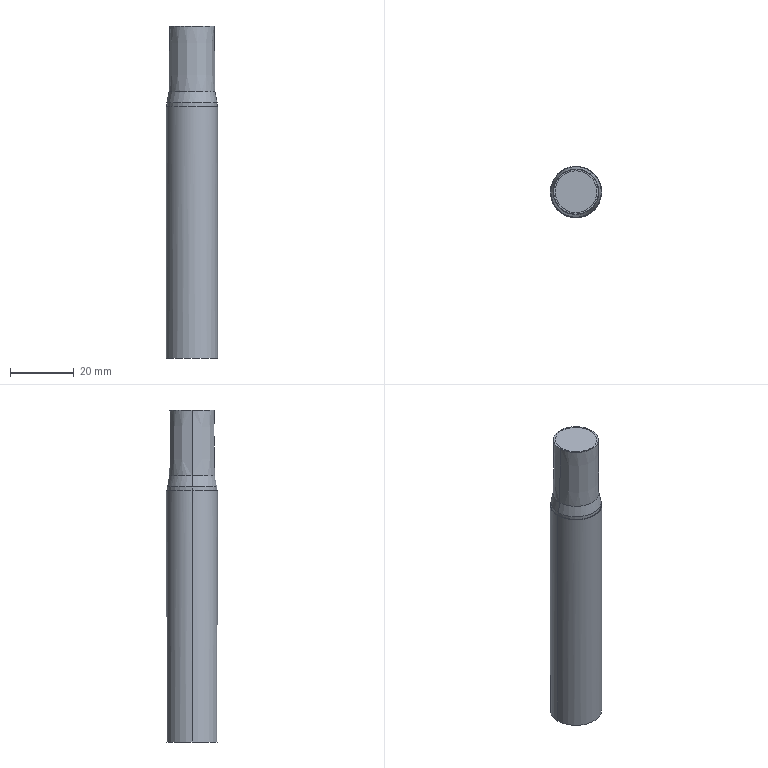Part | Creo | 1 solid | 15 faces | box 16 x 16 x 103.751 mm | volume 19849 mm3 | plane 7 | cone 4 | cylinder 4 | commonest cylinder face diameters 15.678 x2 16 x2
STEP:
#1=CARTESIAN_POINT('',(0.,0.,0.));
#2=DIRECTION('',(0.,0.,1.));
#3=DIRECTION('',(1.,0.,0.));
#4=AXIS2_PLACEMENT_3D('',#1,#2,#3);
#5=CARTESIAN_POINT('',(-38.231,-245.907,-49.693));
#6=VERTEX_POINT('',#5);
#7=CARTESIAN_POINT('',(-31.681,-252.457,-49.728));
#8=VERTEX_POINT('',#7);
#9=CARTESIAN_POINT('',(-37.799,-245.909,-49.693));
#10=CARTESIAN_POINT('',(-36.952,-245.993,-49.694));
#11=CARTESIAN_POINT('',(-35.715,-246.368,-49.696));
#12=CARTESIAN_POINT('',(-34.571,-246.974,-49.699));
#13=CARTESIAN_POINT('',(-33.563,-247.793,-49.703));
#14=CARTESIAN_POINT('',(-32.745,-248.801,-49.709));
#15=CARTESIAN_POINT('',(-32.141,-249.945,-49.715));
#16=CARTESIAN_POINT('',(-31.766,-251.181,-49.721));
#17=CARTESIAN_POINT('',(-31.682,-252.026,-49.726));
#18=B_SPLINE_CURVE_WITH_KNOTS('',3,(#5,#9,#10,#11,#12,#13,#14,#15,#16,#17,#7),.UNSPECIFIED.,.F.,.F.,(4,1,1,1,1,1,1,1,4),(0.,0.125,0.25,0.375,0.5,0.625,0.75,0.875,1.),.UNSPECIFIED.);
#19=EDGE_CURVE('',#6,#8,#18,.T.);
#20=ORIENTED_EDGE('',*,*,#19,.T.);
#21=CARTESIAN_POINT('',(-38.231,-259.008,-49.763));
#22=VERTEX_POINT('',#21);
#23=CARTESIAN_POINT('',(-31.681,-252.457,-49.728));
#24=CARTESIAN_POINT('',(-31.682,-252.889,-49.731));
#25=CARTESIAN_POINT('',(-31.766,-253.736,-49.735));
#26=CARTESIAN_POINT('',(-32.142,-254.974,-49.742));
#27=CARTESIAN_POINT('',(-32.748,-256.118,-49.748));
#28=CARTESIAN_POINT('',(-33.567,-257.126,-49.753));
#29=CARTESIAN_POINT('',(-34.575,-257.944,-49.758));
#30=CARTESIAN_POINT('',(-35.719,-258.548,-49.761));
#31=CARTESIAN_POINT('',(-36.955,-258.923,-49.763));
#32=CARTESIAN_POINT('',(-37.8,-259.007,-49.763));
#33=CARTESIAN_POINT('',(-38.231,-259.008,-49.763));
#34=B_SPLINE_CURVE_WITH_KNOTS('',3,(#23,#24,#25,#26,#27,#28,#29,#30,#31,#32,#33),.UNSPECIFIED.,.F.,.F.,(4,1,1,1,1,1,1,1,4),(0.,0.125,0.25,0.375,0.5,0.625,0.75,0.875,1.),.UNSPECIFIED.);
#35=EDGE_CURVE('',#8,#22,#34,.T.);
#36=ORIENTED_EDGE('',*,*,#35,.T.);
#37=CARTESIAN_POINT('',(-44.782,-252.457,-49.728));
#38=VERTEX_POINT('',#37);
#39=CARTESIAN_POINT('',(-38.664,-259.006,-49.763));
#40=CARTESIAN_POINT('',(-39.51,-258.922,-49.763));
#41=CARTESIAN_POINT('',(-40.748,-258.547,-49.761));
#42=CARTESIAN_POINT('',(-41.892,-257.941,-49.758));
#43=CARTESIAN_POINT('',(-42.9,-257.122,-49.753));
#44=CARTESIAN_POINT('',(-43.718,-256.113,-49.748));
#45=CARTESIAN_POINT('',(-44.322,-254.969,-49.742));
#46=CARTESIAN_POINT('',(-44.697,-253.733,-49.735));
#47=CARTESIAN_POINT('',(-44.78,-252.888,-49.731));
#48=CARTESIAN_POINT('',(-44.782,-252.457,-49.728));
#49=B_SPLINE_CURVE_WITH_KNOTS('',3,(#21,#39,#40,#41,#42,#43,#44,#45,#46,#47,#48),.UNSPECIFIED.,.F.,.F.,(4,1,1,1,1,1,1,1,4),(0.,0.125,0.25,0.375,0.5,0.625,0.75,0.875,1.),.UNSPECIFIED.);
#50=EDGE_CURVE('',#22,#38,#49,.T.);
#51=ORIENTED_EDGE('',*,*,#50,.T.);
#52=CARTESIAN_POINT('',(-44.78,-252.025,-49.726));
#53=CARTESIAN_POINT('',(-44.696,-251.178,-49.721));
#54=CARTESIAN_POINT('',(-44.32,-249.941,-49.715));
#55=CARTESIAN_POINT('',(-43.715,-248.797,-49.709));
#56=CARTESIAN_POINT('',(-42.895,-247.789,-49.703));
#57=CARTESIAN_POINT('',(-41.887,-246.971,-49.699));
#58=CARTESIAN_POINT('',(-40.743,-246.367,-49.696));
#59=CARTESIAN_POINT('',(-39.507,-245.992,-49.694));
#60=CARTESIAN_POINT('',(-38.662,-245.909,-49.693));
#61=CARTESIAN_POINT('',(-38.231,-245.907,-49.693));
#62=B_SPLINE_CURVE_WITH_KNOTS('',3,(#37,#52,#53,#54,#55,#56,#57,#58,#59,#60,#61),.UNSPECIFIED.,.F.,.F.,(4,1,1,1,1,1,1,1,4),(0.,0.125,0.25,0.375,0.5,0.625,0.75,0.875,1.),.UNSPECIFIED.);
#63=EDGE_CURVE('',#38,#6,#62,.T.);
#64=ORIENTED_EDGE('',*,*,#63,.T.);
#65=EDGE_LOOP('',(#20,#36,#51,#64));
#66=FACE_OUTER_BOUND('',#65,.F.);
#67=CARTESIAN_POINT('',(-38.231,-252.458,-49.728));
#68=DIRECTION('',(0.000000109,-0.005365,1.));
#69=DIRECTION('',(1.,0.00000021,-0.000000108));
#70=AXIS2_PLACEMENT_3D('',#67,#68,#69);
#71=PLANE('',#70);
#72=ADVANCED_FACE('',(#66),#71,.T.);
#73=CARTESIAN_POINT('',(-38.231,-259.449,-49.766));
#74=VERTEX_POINT('',#73);
#75=CARTESIAN_POINT('',(-31.239,-252.457,-49.728));
#76=VERTEX_POINT('',#75);
#77=CARTESIAN_POINT('',(-38.231,-259.449,-49.766));
#78=CARTESIAN_POINT('',(-37.649,-259.449,-49.766));
#79=CARTESIAN_POINT('',(-36.621,-259.312,-49.765));
#80=CARTESIAN_POINT('',(-34.891,-258.71,-49.762));
#81=CARTESIAN_POINT('',(-33.188,-257.5,-49.755));
#82=CARTESIAN_POINT('',(-31.978,-255.797,-49.746));
#83=CARTESIAN_POINT('',(-31.377,-254.067,-49.737));
#84=CARTESIAN_POINT('',(-31.239,-253.039,-49.731));
#85=CARTESIAN_POINT('',(-31.239,-252.457,-49.728));
#86=B_SPLINE_CURVE_WITH_KNOTS('',3,(#77,#78,#79,#80,#81,#82,#83,#84,#85),.UNSPECIFIED.,.F.,.F.,(4,1,1,1,1,1,4),(0.,0.125,0.25,0.5,0.75,0.875,1.),.UNSPECIFIED.);
#87=EDGE_CURVE('',#74,#76,#86,.T.);
#88=ORIENTED_EDGE('',*,*,#87,.F.);
#89=CARTESIAN_POINT('',(-45.224,-252.457,-49.728));
#90=VERTEX_POINT('',#89);
#91=CARTESIAN_POINT('',(-45.224,-252.457,-49.728));
#92=CARTESIAN_POINT('',(-45.224,-253.039,-49.731));
#93=CARTESIAN_POINT('',(-45.086,-254.067,-49.737));
#94=CARTESIAN_POINT('',(-44.485,-255.797,-49.746));
#95=CARTESIAN_POINT('',(-43.274,-257.5,-49.755));
#96=CARTESIAN_POINT('',(-41.571,-258.71,-49.762));
#97=CARTESIAN_POINT('',(-39.842,-259.312,-49.765));
#98=CARTESIAN_POINT('',(-38.814,-259.449,-49.766));
#99=B_SPLINE_CURVE_WITH_KNOTS('',3,(#91,#92,#93,#94,#95,#96,#97,#98,#73),.UNSPECIFIED.,.F.,.F.,(4,1,1,1,1,1,4),(0.,0.125,0.25,0.5,0.75,0.875,1.),.UNSPECIFIED.);
#100=EDGE_CURVE('',#90,#74,#99,.T.);
#101=ORIENTED_EDGE('',*,*,#100,.F.);
#102=CARTESIAN_POINT('',(-31.239,-252.457,-49.728));
#103=CARTESIAN_POINT('',(-31.239,-251.633,-49.724));
#104=CARTESIAN_POINT('',(-31.538,-249.852,-49.714));
#105=CARTESIAN_POINT('',(-32.873,-247.782,-49.703));
#106=CARTESIAN_POINT('',(-34.383,-246.56,-49.697));
#107=CARTESIAN_POINT('',(-35.648,-245.909,-49.693));
#108=CARTESIAN_POINT('',(-36.969,-245.538,-49.691));
#109=CARTESIAN_POINT('',(-38.231,-245.428,-49.691));
#110=CARTESIAN_POINT('',(-39.494,-245.538,-49.691));
#111=CARTESIAN_POINT('',(-40.814,-245.909,-49.693));
#112=CARTESIAN_POINT('',(-42.08,-246.56,-49.697));
#113=CARTESIAN_POINT('',(-43.59,-247.782,-49.703));
#114=CARTESIAN_POINT('',(-44.925,-249.852,-49.714));
#115=CARTESIAN_POINT('',(-45.224,-251.633,-49.724));
#116=CARTESIAN_POINT('',(-45.224,-252.457,-49.728));
#117=B_SPLINE_CURVE_WITH_KNOTS('',3,(#102,#103,#104,#105,#106,#107,#108,#109,#110,#111,#112,#113,#114,#115,#116),.UNSPECIFIED.,.F.,.F.,(4,1,1,1,1,1,1,1,1,1,1,1,4),(0.,0.125,0.25,0.3125,0.375,0.4375,0.5,0.5625,0.625,0.6875,0.75,0.875,1.),.UNSPECIFIED.);
#118=EDGE_CURVE('',#76,#90,#117,.T.);
#119=ORIENTED_EDGE('',*,*,#118,.F.);
#120=EDGE_LOOP('',(#88,#101,#119));
#121=FACE_OUTER_BOUND('',#120,.F.);
#122=ORIENTED_EDGE('',*,*,#50,.F.);
#123=ORIENTED_EDGE('',*,*,#35,.F.);
#124=ORIENTED_EDGE('',*,*,#19,.F.);
#125=ORIENTED_EDGE('',*,*,#63,.F.);
#126=EDGE_LOOP('',(#122,#123,#124,#125));
#127=FACE_BOUND('',#126,.F.);
#128=CARTESIAN_POINT('',(-9.454,-218.25,-49.545));
#129=DIRECTION('',(-0.000000109,0.005365,-1.));
#130=DIRECTION('',(0.,1.,0.005365));
#131=AXIS2_PLACEMENT_3D('',#128,#129,#130);
#132=PLANE('',#131);
#133=ADVANCED_FACE('',(#121,#127),#132,.F.);
#134=CARTESIAN_POINT('',(-45.367,-252.457,-70.228));
#135=VERTEX_POINT('',#134);
#136=CARTESIAN_POINT('',(-31.096,-252.457,-70.228));
#137=VERTEX_POINT('',#136);
#138=CARTESIAN_POINT('',(-45.367,-252.457,-70.228));
#139=CARTESIAN_POINT('',(-45.367,-252.924,-70.228));
#140=CARTESIAN_POINT('',(-45.275,-253.858,-70.22));
#141=CARTESIAN_POINT('',(-44.866,-255.205,-70.223));
#142=CARTESIAN_POINT('',(-44.203,-256.447,-70.223));
#143=CARTESIAN_POINT('',(-43.309,-257.535,-70.224));
#144=CARTESIAN_POINT('',(-42.221,-258.428,-70.225));
#145=CARTESIAN_POINT('',(-40.98,-259.092,-70.226));
#146=CARTESIAN_POINT('',(-39.632,-259.5,-70.227));
#147=CARTESIAN_POINT('',(-38.231,-259.638,-70.228));
#148=CARTESIAN_POINT('',(-36.83,-259.5,-70.229));
#149=CARTESIAN_POINT('',(-35.483,-259.092,-70.23));
#150=CARTESIAN_POINT('',(-34.242,-258.428,-70.231));
#151=CARTESIAN_POINT('',(-33.153,-257.535,-70.231));
#152=CARTESIAN_POINT('',(-32.26,-256.447,-70.232));
#153=CARTESIAN_POINT('',(-31.597,-255.205,-70.232));
#154=CARTESIAN_POINT('',(-31.188,-253.858,-70.235));
#155=CARTESIAN_POINT('',(-31.096,-252.924,-70.228));
#156=CARTESIAN_POINT('',(-31.096,-252.457,-70.228));
#157=B_SPLINE_CURVE_WITH_KNOTS('',3,(#138,#139,#140,#141,#142,#143,#144,#145,#146,#147,#148,#149,#150,#151,#152,#153,#154,#155,#156),.UNSPECIFIED.,.F.,.F.,(4,1,1,1,1,1,1,1,1,1,1,1,1,1,1,1,4),(0.,0.0625,0.125,0.1875,0.25,0.3125,0.375,0.4375,0.5,0.5625,0.625,0.6875,0.75,0.8125,0.875,0.9375,1.),.UNSPECIFIED.);
#158=EDGE_CURVE('',#135,#137,#157,.T.);
#159=ORIENTED_EDGE('',*,*,#158,.F.);
#160=CARTESIAN_POINT('',(-45.224,-252.457,-49.728));
#161=DIRECTION('',(-0.007005,0.,-1.));
#162=VECTOR('',#161,20.5);
#163=LINE('',#160,#162);
#164=EDGE_CURVE('',#90,#135,#163,.T.);
#165=ORIENTED_EDGE('',*,*,#164,.F.);
#166=ORIENTED_EDGE('',*,*,#100,.T.);
#167=ORIENTED_EDGE('',*,*,#87,.T.);
#168=CARTESIAN_POINT('',(-31.239,-252.457,-49.728));
#169=DIRECTION('',(0.006958,0.,-1.));
#170=VECTOR('',#169,20.5);
#171=LINE('',#168,#170);
#172=EDGE_CURVE('',#76,#137,#171,.T.);
#173=ORIENTED_EDGE('',*,*,#172,.T.);
#174=EDGE_LOOP('',(#159,#165,#166,#167,#173));
#175=FACE_OUTER_BOUND('',#174,.F.);
#176=CARTESIAN_POINT('',(-38.231,-252.457,-59.981));
#177=DIRECTION('',(0.,0.,-1.));
#178=DIRECTION('',(1.,0.,0.));
#179=AXIS2_PLACEMENT_3D('',#176,#177,#178);
#180=CONICAL_SURFACE('',#179,7.064,0.4);
#181=ADVANCED_FACE('',(#175),#180,.T.);
#182=ORIENTED_EDGE('',*,*,#158,.T.);
#183=CARTESIAN_POINT('',(-30.393,-252.457,-73.745));
#184=VERTEX_POINT('',#183);
#185=CARTESIAN_POINT('',(-31.096,-252.457,-70.228));
#186=DIRECTION('',(0.1961,0.,-0.9806));
#187=VECTOR('',#186,3.587);
#188=LINE('',#185,#187);
#189=EDGE_CURVE('',#137,#184,#188,.T.);
#190=ORIENTED_EDGE('',*,*,#189,.T.);
#191=CARTESIAN_POINT('',(-46.07,-252.457,-73.742));
#192=VERTEX_POINT('',#191);
#193=CARTESIAN_POINT('',(-38.231,-252.457,-73.745));
#194=DIRECTION('',(0.,0.,1.));
#195=DIRECTION('',(-1.,0.,0.));
#196=AXIS2_PLACEMENT_3D('',#193,#194,#195);
#197=CIRCLE('',#196,7.839);
#198=EDGE_CURVE('',#192,#184,#197,.T.);
#199=ORIENTED_EDGE('',*,*,#198,.F.);
#200=CARTESIAN_POINT('',(-45.367,-252.457,-70.228));
#201=DIRECTION('',(-0.1961,0.,-0.9806));
#202=VECTOR('',#201,3.584);
#203=LINE('',#200,#202);
#204=EDGE_CURVE('',#135,#192,#203,.T.);
#205=ORIENTED_EDGE('',*,*,#204,.F.);
#206=EDGE_LOOP('',(#182,#190,#199,#205));
#207=FACE_OUTER_BOUND('',#206,.F.);
#208=CARTESIAN_POINT('',(-38.232,-252.457,-71.987));
#209=DIRECTION('',(-0.00002709,0.,-1.));
#210=DIRECTION('',(1.,0.,-0.00002709));
#211=AXIS2_PLACEMENT_3D('',#208,#209,#210);
#212=CONICAL_SURFACE('',#211,7.487,11.31);
#213=ADVANCED_FACE('',(#207),#212,.T.);
#214=CARTESIAN_POINT('',(-31.096,-252.457,-70.228));
#215=CARTESIAN_POINT('',(-31.096,-251.99,-70.228));
#216=CARTESIAN_POINT('',(-31.188,-251.056,-70.235));
#217=CARTESIAN_POINT('',(-31.597,-249.709,-70.232));
#218=CARTESIAN_POINT('',(-32.26,-248.467,-70.232));
#219=CARTESIAN_POINT('',(-33.153,-247.379,-70.231));
#220=CARTESIAN_POINT('',(-34.242,-246.486,-70.231));
#221=CARTESIAN_POINT('',(-35.483,-245.822,-70.23));
#222=CARTESIAN_POINT('',(-36.83,-245.413,-70.229));
#223=CARTESIAN_POINT('',(-38.231,-245.275,-70.228));
#224=CARTESIAN_POINT('',(-39.632,-245.413,-70.227));
#225=CARTESIAN_POINT('',(-40.98,-245.822,-70.226));
#226=CARTESIAN_POINT('',(-42.221,-246.486,-70.225));
#227=CARTESIAN_POINT('',(-43.309,-247.379,-70.224));
#228=CARTESIAN_POINT('',(-44.203,-248.467,-70.223));
#229=CARTESIAN_POINT('',(-44.866,-249.709,-70.223));
#230=CARTESIAN_POINT('',(-45.275,-251.056,-70.22));
#231=CARTESIAN_POINT('',(-45.367,-251.99,-70.228));
#232=CARTESIAN_POINT('',(-45.367,-252.457,-70.228));
#233=B_SPLINE_CURVE_WITH_KNOTS('',3,(#214,#215,#216,#217,#218,#219,#220,#221,#222,#223,#224,#225,#226,#227,#228,#229,#230,#231,#232),.UNSPECIFIED.,.F.,.F.,(4,1,1,1,1,1,1,1,1,1,1,1,1,1,1,1,4),(0.,0.0625,0.125,0.1875,0.25,0.3125,0.375,0.4375,0.5,0.5625,0.625,0.6875,0.75,0.8125,0.875,0.9375,1.),.UNSPECIFIED.);
#234=EDGE_CURVE('',#137,#135,#233,.T.);
#235=ORIENTED_EDGE('',*,*,#234,.T.);
#236=ORIENTED_EDGE('',*,*,#204,.T.);
#237=CARTESIAN_POINT('',(-38.231,-252.457,-73.745));
#238=DIRECTION('',(0.,0.,1.));
#239=DIRECTION('',(1.,0.,0.));
#240=AXIS2_PLACEMENT_3D('',#237,#238,#239);
#241=CIRCLE('',#240,7.839);
#242=EDGE_CURVE('',#184,#192,#241,.T.);
#243=ORIENTED_EDGE('',*,*,#242,.F.);
#244=ORIENTED_EDGE('',*,*,#189,.F.);
#245=EDGE_LOOP('',(#235,#236,#243,#244));
#246=FACE_OUTER_BOUND('',#245,.F.);
#247=CARTESIAN_POINT('',(-38.232,-252.457,-71.987));
#248=DIRECTION('',(-0.00002709,0.,-1.));
#249=DIRECTION('',(1.,0.,-0.00002709));
#250=AXIS2_PLACEMENT_3D('',#247,#248,#249);
#251=CONICAL_SURFACE('',#250,7.487,11.31);
#252=ADVANCED_FACE('',(#246),#251,.T.);
#253=ORIENTED_EDGE('',*,*,#234,.F.);
#254=ORIENTED_EDGE('',*,*,#172,.F.);
#255=ORIENTED_EDGE('',*,*,#118,.T.);
#256=ORIENTED_EDGE('',*,*,#164,.T.);
#257=EDGE_LOOP('',(#253,#254,#255,#256));
#258=FACE_OUTER_BOUND('',#257,.F.);
#259=CARTESIAN_POINT('',(-38.231,-252.457,-59.962));
#260=DIRECTION('',(0.,0.,-1.));
#261=DIRECTION('',(1.,0.,0.));
#262=AXIS2_PLACEMENT_3D('',#259,#260,#261);
#263=CONICAL_SURFACE('',#262,7.064,0.4);
#264=ADVANCED_FACE('',(#258),#263,.T.);
#265=CARTESIAN_POINT('',(-46.07,-252.457,-74.75));
#266=VERTEX_POINT('',#265);
#267=CARTESIAN_POINT('',(-30.392,-252.457,-74.75));
#268=VERTEX_POINT('',#267);
#269=CARTESIAN_POINT('',(-38.231,-252.457,-74.75));
#270=DIRECTION('',(0.,0.,-1.));
#271=DIRECTION('',(-1.,0.,0.));
#272=AXIS2_PLACEMENT_3D('',#269,#270,#271);
#273=CIRCLE('',#272,7.839);
#274=EDGE_CURVE('',#266,#268,#273,.T.);
#275=ORIENTED_EDGE('',*,*,#274,.T.);
#276=CARTESIAN_POINT('',(-30.392,-252.457,-74.75));
#277=DIRECTION('',(-0.0005284,0.,1.));
#278=VECTOR('',#277,1.005);
#279=LINE('',#276,#278);
#280=EDGE_CURVE('',#268,#184,#279,.T.);
#281=ORIENTED_EDGE('',*,*,#280,.T.);
#282=ORIENTED_EDGE('',*,*,#242,.T.);
#283=CARTESIAN_POINT('',(-46.07,-252.457,-74.75));
#284=DIRECTION('',(0.,0.,1.));
#285=VECTOR('',#284,1.008);
#286=LINE('',#283,#285);
#287=EDGE_CURVE('',#266,#192,#286,.T.);
#288=ORIENTED_EDGE('',*,*,#287,.F.);
#289=EDGE_LOOP('',(#275,#281,#282,#288));
#290=FACE_OUTER_BOUND('',#289,.F.);
#291=CARTESIAN_POINT('',(-38.231,-252.457,-74.75));
#292=DIRECTION('',(0.,0.,1.));
#293=DIRECTION('',(1.,0.,0.));
#294=AXIS2_PLACEMENT_3D('',#291,#292,#293);
#295=CYLINDRICAL_SURFACE('',#294,7.839);
#296=ADVANCED_FACE('',(#290),#295,.T.);
#297=CARTESIAN_POINT('',(-38.235,-260.444,-74.75));
#298=VERTEX_POINT('',#297);
#299=CARTESIAN_POINT('',(-46.219,-252.457,-74.75));
#300=VERTEX_POINT('',#299);
#301=CARTESIAN_POINT('',(-38.764,-260.443,-74.75));
#302=CARTESIAN_POINT('',(-39.799,-260.341,-74.75));
#303=CARTESIAN_POINT('',(-41.312,-259.882,-74.75));
#304=CARTESIAN_POINT('',(-42.699,-259.14,-74.75));
#305=CARTESIAN_POINT('',(-43.916,-258.141,-74.75));
#306=CARTESIAN_POINT('',(-44.914,-256.925,-74.75));
#307=CARTESIAN_POINT('',(-45.657,-255.537,-74.75));
#308=CARTESIAN_POINT('',(-46.116,-254.026,-74.75));
#309=CARTESIAN_POINT('',(-46.217,-252.988,-74.75));
#310=B_SPLINE_CURVE_WITH_KNOTS('',3,(#297,#301,#302,#303,#304,#305,#306,#307,#308,#309,#299),.UNSPECIFIED.,.F.,.F.,(4,1,1,1,1,1,1,1,4),(0.,0.125,0.25,0.375,0.5,0.625,0.75,0.875,1.),.UNSPECIFIED.);
#311=EDGE_CURVE('',#298,#300,#310,.T.);
#312=ORIENTED_EDGE('',*,*,#311,.T.);
#313=CARTESIAN_POINT('',(-43.892,-246.821,-74.75));
#314=VERTEX_POINT('',#313);
#315=CARTESIAN_POINT('',(-46.219,-252.457,-74.75));
#316=CARTESIAN_POINT('',(-46.218,-251.929,-74.75));
#317=CARTESIAN_POINT('',(-46.117,-250.896,-74.75));
#318=CARTESIAN_POINT('',(-45.662,-249.389,-74.75));
#319=CARTESIAN_POINT('',(-44.921,-248.,-74.75));
#320=CARTESIAN_POINT('',(-44.263,-247.196,-74.75));
#321=B_SPLINE_CURVE_WITH_KNOTS('',3,(#315,#316,#317,#318,#319,#320,#313),.UNSPECIFIED.,.F.,.F.,(4,1,1,1,4),(0.,0.25,0.5,0.75,1.),.UNSPECIFIED.);
#322=EDGE_CURVE('',#300,#314,#321,.T.);
#323=ORIENTED_EDGE('',*,*,#322,.T.);
#324=CARTESIAN_POINT('',(-38.435,-244.459,-74.75));
#325=VERTEX_POINT('',#324);
#326=CARTESIAN_POINT('',(-43.892,-246.821,-74.75));
#327=CARTESIAN_POINT('',(-43.565,-246.501,-74.75));
#328=CARTESIAN_POINT('',(-42.888,-245.927,-74.75));
#329=CARTESIAN_POINT('',(-41.786,-245.273,-74.75));
#330=CARTESIAN_POINT('',(-40.65,-244.808,-74.75));
#331=CARTESIAN_POINT('',(-39.481,-244.548,-74.75));
#332=CARTESIAN_POINT('',(-38.777,-244.472,-74.75));
#333=CARTESIAN_POINT('',(-38.435,-244.462,-74.75));
#334=B_SPLINE_CURVE_WITH_KNOTS('',3,(#326,#327,#328,#329,#330,#331,#332,#333),.UNSPECIFIED.,.F.,.F.,(4,1,1,1,1,4),(0.,0.2,0.4,0.6,0.8,1.),.UNSPECIFIED.);
#335=EDGE_CURVE('',#314,#325,#334,.T.);
#336=ORIENTED_EDGE('',*,*,#335,.T.);
#337=CARTESIAN_POINT('',(-38.231,-244.47,-74.75));
#338=VERTEX_POINT('',#337);
#339=CARTESIAN_POINT('',(-38.435,-244.462,-74.75));
#340=CARTESIAN_POINT('',(-38.401,-244.465,-74.75));
#341=CARTESIAN_POINT('',(-38.333,-244.47,-74.75));
#342=CARTESIAN_POINT('',(-38.265,-244.47,-74.75));
#343=CARTESIAN_POINT('',(-38.231,-244.47,-74.75));
#344=B_SPLINE_CURVE_WITH_KNOTS('',3,(#339,#340,#341,#342,#343),.UNSPECIFIED.,.F.,.F.,(4,1,4),(0.,0.5,1.),.UNSPECIFIED.);
#345=EDGE_CURVE('',#325,#338,#344,.T.);
#346=ORIENTED_EDGE('',*,*,#345,.T.);
#347=CARTESIAN_POINT('',(-37.749,-244.478,-74.75));
#348=VERTEX_POINT('',#347);
#349=CARTESIAN_POINT('',(-38.153,-244.468,-74.75));
#350=CARTESIAN_POINT('',(-37.995,-244.469,-74.75));
#351=CARTESIAN_POINT('',(-37.832,-244.473,-74.75));
#352=B_SPLINE_CURVE_WITH_KNOTS('',3,(#337,#349,#350,#351,#347),.UNSPECIFIED.,.F.,.F.,(4,1,4),(0.,0.5,1.),.UNSPECIFIED.);
#353=EDGE_CURVE('',#338,#348,#352,.T.);
#354=ORIENTED_EDGE('',*,*,#353,.T.);
#355=CARTESIAN_POINT('',(-30.39,-250.872,-74.75));
#356=VERTEX_POINT('',#355);
#357=CARTESIAN_POINT('',(-37.749,-244.478,-74.75));
#358=CARTESIAN_POINT('',(-37.409,-244.494,-74.75));
#359=CARTESIAN_POINT('',(-36.703,-244.593,-74.75));
#360=CARTESIAN_POINT('',(-35.536,-244.903,-74.75));
#361=CARTESIAN_POINT('',(-34.362,-245.439,-74.75));
#362=CARTESIAN_POINT('',(-33.254,-246.168,-74.75));
#363=CARTESIAN_POINT('',(-32.271,-247.083,-74.75));
#364=CARTESIAN_POINT('',(-31.437,-248.189,-74.75));
#365=CARTESIAN_POINT('',(-30.763,-249.492,-74.75));
#366=CARTESIAN_POINT('',(-30.489,-250.4,-74.75));
#367=CARTESIAN_POINT('',(-30.39,-250.872,-74.75));
#368=B_SPLINE_CURVE_WITH_KNOTS('',3,(#357,#358,#359,#360,#361,#362,#363,#364,#365,#366,#367),.UNSPECIFIED.,.F.,.F.,(4,1,1,1,1,1,1,1,4),(0.,0.125,0.25,0.375,0.5,0.625,0.75,0.875,1.),.UNSPECIFIED.);
#369=EDGE_CURVE('',#348,#356,#368,.T.);
#370=ORIENTED_EDGE('',*,*,#369,.T.);
#371=CARTESIAN_POINT('',(-30.244,-252.466,-74.75));
#372=VERTEX_POINT('',#371);
#373=CARTESIAN_POINT('',(-30.39,-250.872,-74.75));
#374=CARTESIAN_POINT('',(-30.339,-251.131,-74.75));
#375=CARTESIAN_POINT('',(-30.263,-251.655,-74.75));
#376=CARTESIAN_POINT('',(-30.241,-252.193,-74.75));
#377=CARTESIAN_POINT('',(-30.244,-252.466,-74.75));
#378=B_SPLINE_CURVE_WITH_KNOTS('',3,(#373,#374,#375,#376,#377),.UNSPECIFIED.,.F.,.F.,(4,1,4),(0.,0.5,1.),.UNSPECIFIED.);
#379=EDGE_CURVE('',#356,#372,#378,.T.);
#380=ORIENTED_EDGE('',*,*,#379,.T.);
#381=CARTESIAN_POINT('',(-30.244,-252.992,-74.75));
#382=CARTESIAN_POINT('',(-30.345,-254.024,-74.75));
#383=CARTESIAN_POINT('',(-30.804,-255.539,-74.75));
#384=CARTESIAN_POINT('',(-31.547,-256.925,-74.75));
#385=CARTESIAN_POINT('',(-32.546,-258.142,-74.75));
#386=CARTESIAN_POINT('',(-33.763,-259.14,-74.75));
#387=CARTESIAN_POINT('',(-35.15,-259.883,-74.75));
#388=CARTESIAN_POINT('',(-36.662,-260.341,-74.75));
#389=CARTESIAN_POINT('',(-37.702,-260.443,-74.75));
#390=CARTESIAN_POINT('',(-38.235,-260.444,-74.75));
#391=B_SPLINE_CURVE_WITH_KNOTS('',3,(#371,#381,#382,#383,#384,#385,#386,#387,#388,#389,#390),.UNSPECIFIED.,.F.,.F.,(4,1,1,1,1,1,1,1,4),(0.,0.125,0.25,0.375,0.5,0.625,0.75,0.875,1.),.UNSPECIFIED.);
#392=EDGE_CURVE('',#372,#298,#391,.T.);
#393=ORIENTED_EDGE('',*,*,#392,.T.);
#394=EDGE_LOOP('',(#312,#323,#336,#346,#354,#370,#380,#393));
#395=FACE_OUTER_BOUND('',#394,.F.);
#396=CARTESIAN_POINT('',(-30.599,-254.247,-74.75));
#397=VERTEX_POINT('',#396);
#398=CARTESIAN_POINT('',(-38.231,-252.457,-74.75));
#399=DIRECTION('',(0.,0.,-1.));
#400=DIRECTION('',(0.9736,-0.2283,0.));
#401=AXIS2_PLACEMENT_3D('',#398,#399,#400);
#402=CIRCLE('',#401,7.839);
#403=EDGE_CURVE('',#397,#266,#402,.T.);
#404=ORIENTED_EDGE('',*,*,#403,.F.);
#405=CARTESIAN_POINT('',(-38.231,-252.457,-74.75));
#406=DIRECTION('',(0.,0.,-1.));
#407=DIRECTION('',(1.,0.,0.));
#408=AXIS2_PLACEMENT_3D('',#405,#406,#407);
#409=CIRCLE('',#408,7.839);
#410=EDGE_CURVE('',#268,#397,#409,.T.);
#411=ORIENTED_EDGE('',*,*,#410,.F.);
#412=ORIENTED_EDGE('',*,*,#274,.F.);
#413=EDGE_LOOP('',(#404,#411,#412));
#414=FACE_BOUND('',#413,.F.);
#415=CARTESIAN_POINT('',(-41.052,-251.284,-74.75));
#416=DIRECTION('',(-0.00001194,0.000002801,1.));
#417=DIRECTION('',(1.,0.,0.00001194));
#418=AXIS2_PLACEMENT_3D('',#415,#416,#417);
#419=PLANE('',#418);
#420=ADVANCED_FACE('',(#395,#414),#419,.T.);
#421=ORIENTED_EDGE('',*,*,#410,.T.);
#422=ORIENTED_EDGE('',*,*,#403,.T.);
#423=ORIENTED_EDGE('',*,*,#287,.T.);
#424=ORIENTED_EDGE('',*,*,#198,.T.);
#425=ORIENTED_EDGE('',*,*,#280,.F.);
#426=EDGE_LOOP('',(#421,#422,#423,#424,#425));
#427=FACE_OUTER_BOUND('',#426,.F.);
#428=CARTESIAN_POINT('',(-38.231,-252.457,-74.75));
#429=DIRECTION('',(0.,0.,1.));
#430=DIRECTION('',(1.,0.,0.));
#431=AXIS2_PLACEMENT_3D('',#428,#429,#430);
#432=CYLINDRICAL_SURFACE('',#431,7.839);
#433=ADVANCED_FACE('',(#427),#432,.T.);
#434=CARTESIAN_POINT('',(-46.231,-252.457,-74.75));
#435=VERTEX_POINT('',#434);
#436=CARTESIAN_POINT('',(-38.231,-252.457,-74.75));
#437=DIRECTION('',(0.,0.,1.));
#438=DIRECTION('',(-0.02548,0.9997,0.));
#439=AXIS2_PLACEMENT_3D('',#436,#437,#438);
#440=CIRCLE('',#439,8.);
#441=EDGE_CURVE('',#325,#435,#440,.T.);
#442=ORIENTED_EDGE('',*,*,#441,.F.);
#443=ORIENTED_EDGE('',*,*,#335,.F.);
#444=ORIENTED_EDGE('',*,*,#322,.F.);
#445=ORIENTED_EDGE('',*,*,#311,.F.);
#446=ORIENTED_EDGE('',*,*,#392,.F.);
#447=ORIENTED_EDGE('',*,*,#379,.F.);
#448=CARTESIAN_POINT('',(-30.231,-252.457,-74.75));
#449=VERTEX_POINT('',#448);
#450=CARTESIAN_POINT('',(-38.231,-252.457,-74.75));
#451=DIRECTION('',(0.,0.,1.));
#452=DIRECTION('',(1.,0.,0.));
#453=AXIS2_PLACEMENT_3D('',#450,#451,#452);
#454=CIRCLE('',#453,8.);
#455=EDGE_CURVE('',#449,#356,#454,.T.);
#456=ORIENTED_EDGE('',*,*,#455,.F.);
#457=CARTESIAN_POINT('',(-38.231,-252.457,-74.75));
#458=DIRECTION('',(0.,0.,1.));
#459=DIRECTION('',(-1.,0.,0.));
#460=AXIS2_PLACEMENT_3D('',#457,#458,#459);
#461=CIRCLE('',#460,8.);
#462=EDGE_CURVE('',#435,#449,#461,.T.);
#463=ORIENTED_EDGE('',*,*,#462,.F.);
#464=EDGE_LOOP('',(#442,#443,#444,#445,#446,#447,#456,#463));
#465=FACE_OUTER_BOUND('',#464,.F.);
#466=CARTESIAN_POINT('',(-78.831,-266.882,-74.75));
#467=DIRECTION('',(0.,0.,-1.));
#468=DIRECTION('',(-1.,0.,0.));
#469=AXIS2_PLACEMENT_3D('',#466,#467,#468);
#470=PLANE('',#469);
#471=ADVANCED_FACE('',(#465),#470,.F.);
#472=ORIENTED_EDGE('',*,*,#369,.F.);
#473=CARTESIAN_POINT('',(-38.231,-252.457,-74.75));
#474=DIRECTION('',(0.,0.,1.));
#475=DIRECTION('',(0.9802,0.1981,0.));
#476=AXIS2_PLACEMENT_3D('',#473,#474,#475);
#477=CIRCLE('',#476,8.);
#478=EDGE_CURVE('',#356,#348,#477,.T.);
#479=ORIENTED_EDGE('',*,*,#478,.F.);
#480=EDGE_LOOP('',(#472,#479));
#481=FACE_OUTER_BOUND('',#480,.F.);
#482=CARTESIAN_POINT('',(-78.831,-266.882,-74.75));
#483=DIRECTION('',(0.,0.,-1.));
#484=DIRECTION('',(-1.,0.,0.));
#485=AXIS2_PLACEMENT_3D('',#482,#483,#484);
#486=PLANE('',#485);
#487=ADVANCED_FACE('',(#481),#486,.F.);
#488=ORIENTED_EDGE('',*,*,#353,.F.);
#489=ORIENTED_EDGE('',*,*,#345,.F.);
#490=CARTESIAN_POINT('',(-38.231,-252.457,-74.75));
#491=DIRECTION('',(0.,0.,1.));
#492=DIRECTION('',(0.06035,0.9982,0.));
#493=AXIS2_PLACEMENT_3D('',#490,#491,#492);
#494=CIRCLE('',#493,8.);
#495=EDGE_CURVE('',#348,#325,#494,.T.);
#496=ORIENTED_EDGE('',*,*,#495,.F.);
#497=EDGE_LOOP('',(#488,#489,#496));
#498=FACE_OUTER_BOUND('',#497,.F.);
#499=CARTESIAN_POINT('',(-78.831,-266.882,-74.75));
#500=DIRECTION('',(0.,0.,-1.));
#501=DIRECTION('',(-1.,0.,0.));
#502=AXIS2_PLACEMENT_3D('',#499,#500,#501);
#503=PLANE('',#502);
#504=ADVANCED_FACE('',(#498),#503,.F.);
#505=CARTESIAN_POINT('',(-46.231,-252.457,-153.441));
#506=VERTEX_POINT('',#505);
#507=CARTESIAN_POINT('',(-30.231,-252.457,-153.441));
#508=VERTEX_POINT('',#507);
#509=CARTESIAN_POINT('',(-38.231,-252.457,-153.441));
#510=DIRECTION('',(0.,0.,-1.));
#511=DIRECTION('',(-1.,0.,0.));
#512=AXIS2_PLACEMENT_3D('',#509,#510,#511);
#513=CIRCLE('',#512,8.);
#514=EDGE_CURVE('',#506,#508,#513,.T.);
#515=ORIENTED_EDGE('',*,*,#514,.T.);
#516=CARTESIAN_POINT('',(-30.231,-252.457,-74.75));
#517=DIRECTION('',(0.,0.,-1.));
#518=VECTOR('',#517,78.691);
#519=LINE('',#516,#518);
#520=EDGE_CURVE('',#449,#508,#519,.T.);
#521=ORIENTED_EDGE('',*,*,#520,.F.);
#522=ORIENTED_EDGE('',*,*,#455,.T.);
#523=ORIENTED_EDGE('',*,*,#478,.T.);
#524=ORIENTED_EDGE('',*,*,#495,.T.);
#525=ORIENTED_EDGE('',*,*,#441,.T.);
#526=CARTESIAN_POINT('',(-46.231,-252.457,-74.75));
#527=DIRECTION('',(0.,0.,-1.));
#528=VECTOR('',#527,78.691);
#529=LINE('',#526,#528);
#530=EDGE_CURVE('',#435,#506,#529,.T.);
#531=ORIENTED_EDGE('',*,*,#530,.T.);
#532=EDGE_LOOP('',(#515,#521,#522,#523,#524,#525,#531));
#533=FACE_OUTER_BOUND('',#532,.F.);
#534=CARTESIAN_POINT('',(-38.231,-252.457,508.193));
#535=DIRECTION('',(0.,0.,-1.));
#536=DIRECTION('',(-1.,0.,0.));
#537=AXIS2_PLACEMENT_3D('',#534,#535,#536);
#538=CYLINDRICAL_SURFACE('',#537,8.);
#539=ADVANCED_FACE('',(#533),#538,.T.);
#540=ORIENTED_EDGE('',*,*,#514,.F.);
#541=CARTESIAN_POINT('',(-38.231,-252.457,-153.441));
#542=DIRECTION('',(0.,0.,-1.));
#543=DIRECTION('',(1.,0.,0.));
#544=AXIS2_PLACEMENT_3D('',#541,#542,#543);
#545=CIRCLE('',#544,8.);
#546=EDGE_CURVE('',#508,#506,#545,.T.);
#547=ORIENTED_EDGE('',*,*,#546,.F.);
#548=EDGE_LOOP('',(#540,#547));
#549=FACE_OUTER_BOUND('',#548,.F.);
#550=CARTESIAN_POINT('',(5.725,319.968,-153.441));
#551=DIRECTION('',(0.,0.,-1.));
#552=DIRECTION('',(-1.,0.,0.));
#553=AXIS2_PLACEMENT_3D('',#550,#551,#552);
#554=PLANE('',#553);
#555=ADVANCED_FACE('',(#549),#554,.T.);
#556=ORIENTED_EDGE('',*,*,#546,.T.);
#557=ORIENTED_EDGE('',*,*,#530,.F.);
#558=ORIENTED_EDGE('',*,*,#462,.T.);
#559=ORIENTED_EDGE('',*,*,#520,.T.);
#560=EDGE_LOOP('',(#556,#557,#558,#559));
#561=FACE_OUTER_BOUND('',#560,.F.);
#562=CARTESIAN_POINT('',(-38.231,-252.457,508.193));
#563=DIRECTION('',(0.,0.,-1.));
#564=DIRECTION('',(-1.,0.,0.));
#565=AXIS2_PLACEMENT_3D('',#562,#563,#564);
#566=CYLINDRICAL_SURFACE('',#565,8.);
#567=ADVANCED_FACE('',(#561),#566,.T.);
#568=CLOSED_SHELL('',(#72,#133,#181,#213,#252,#264,#296,#420,#433,#471,#487,#504,#539,#555,#567));
#569=MANIFOLD_SOLID_BREP('',#568);
#570=(LENGTH_UNIT()NAMED_UNIT(*)SI_UNIT(.MILLI.,.METRE.));
#571=UNCERTAINTY_MEASURE_WITH_UNIT(LENGTH_MEASURE(0.01062),#570,'','');
#572=(NAMED_UNIT(*)PLANE_ANGLE_UNIT()SI_UNIT($,.RADIAN.));
#573=PLANE_ANGLE_MEASURE_WITH_UNIT(PLANE_ANGLE_MEASURE(0.01745),#572);
#574=(CONVERSION_BASED_UNIT('DEGREE',#573)NAMED_UNIT(*)PLANE_ANGLE_UNIT());
#575=(NAMED_UNIT(*)SI_UNIT($,.STERADIAN.)SOLID_ANGLE_UNIT());
#576=(GEOMETRIC_REPRESENTATION_CONTEXT(3)GLOBAL_UNCERTAINTY_ASSIGNED_CONTEXT((#571))GLOBAL_UNIT_ASSIGNED_CONTEXT((#570,#574,#575))REPRESENTATION_CONTEXT('',''));
#577=ADVANCED_BREP_SHAPE_REPRESENTATION('',(#4,#569),#576);